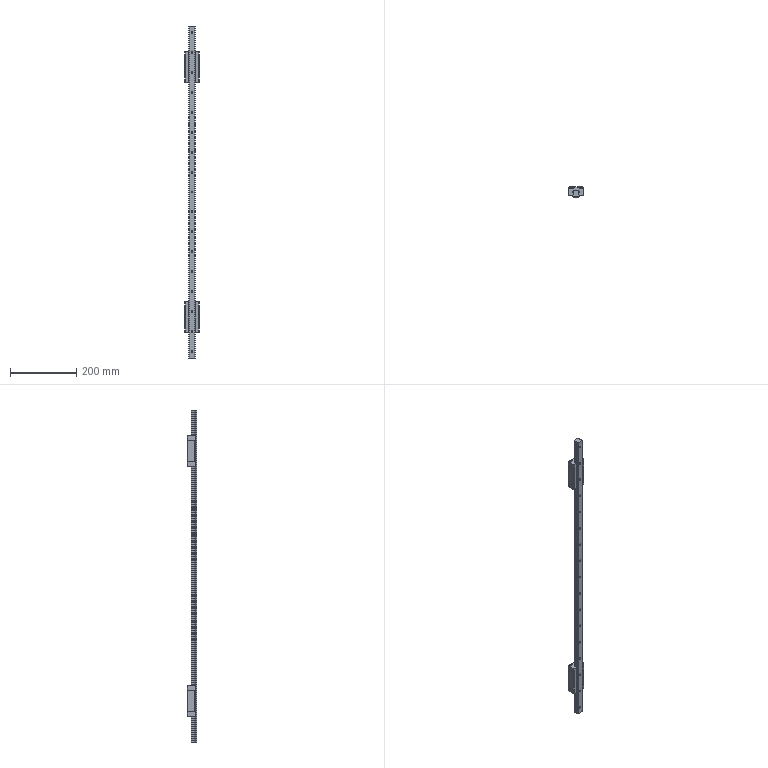Part | SolidWorks | 3 solids | 883 faces | box 44 x 30 x 1000 mm | volume 445090 mm3 | plane 609 | cylinder 154 | spline 120 | commonest cylinder face diameters 1 x36 6 x34 9.5 x34 2 x22 5 x16 4.06 x12